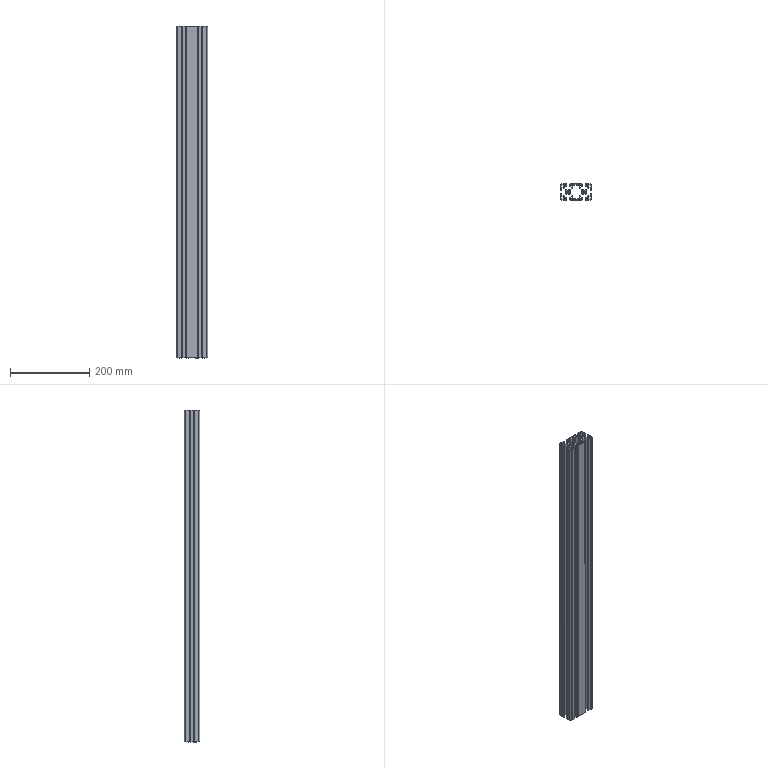Part | STEP file | HJLE-8-4080-S-OO_LE0724151524 | 1 solid | 286 faces | box 80 x 40 x 840 mm | volume 675539 mm3 | cylinder 144 | plane 142 | commonest cylinder face diameters 0.6 x48 2 x36 4 x28 0.4 x12 5 x4 6 x4